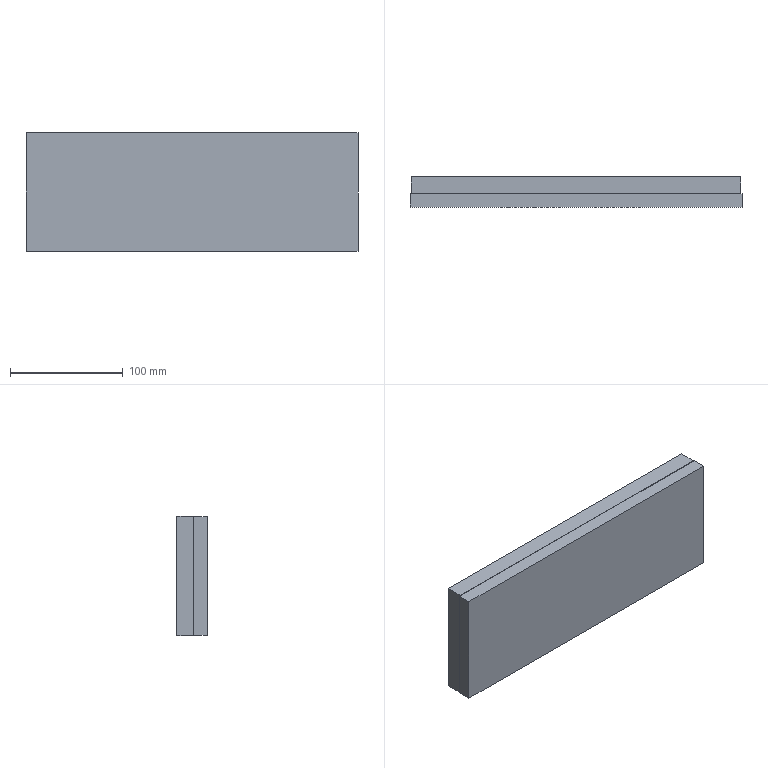NC program | NX | posted with a generic post | part box 295 x 27 x 106 mm
Lines 1 to 1810 of 7486, first 1519 of 1788 lines:
N10 G17 G21 G94 G90
(DRILLING , TOOL : DK-D8点孔)
N12 T04 M6
N14 G53
N16 G17 G0 G90 X102. Y-38.5 S2000 M3
N18 G43 Z20. H4
N20 G94 G81 G99 Z-3. F200. R3.
N22 Y0.
N24 Y38.5
N26 X-117. Y38.616
N28 Y0.
N30 G80
N32 G0 X-117. Y0. Z20.
N34 M5
(DRILLING_COPY , TOOL : D05钻头)
N36 T05 M6
N38 G53
N40 G17 G0 G90 X102. Y-38.5 S2000 M3
N42 G43 Z20. H5
N44 G94 G81 G99 Z-14. F200. R3.
N46 Y38.5
N48 X-117. Y0.
N50 G80
N52 G0 X-117. Y0. Z20.
(DRILLING_COPY_1 , TOOL : D05钻头)
N54 Y38.616
N56 G81 Z-7. F200. R3.
N58 X102. Y0.
N60 G80
N62 G0 X102. Y0. Z20.
N64 M5
(FLOOR_WALL_1 , TOOL : D63光面)
N66 T01 M6
N68 G54
N70 G17 G0 G90 X222.5 Y-30.25 S4000 M3
N72 G43 Z4.525 H1
N74 G94 G1 Z1.525 F1000.
N76 X212.5
N78 X-135.5
N80 Y-1.725
N82 X212.5
N84 Y26.8
N86 X-135.5
N88 X-145.5
N90 Z4.525
N92 G0 Z5.
N94 X222.5 Y-30.25
N96 Z4.05
N98 G1 Z1.05
N100 X212.5
N102 X-135.5
N104 Y-1.725
N106 X212.5
N108 Y26.8
N110 X-135.5
N112 X-145.5
N114 Z4.05
N116 G0 Z5.
N118 X222.5 Y-30.25
N120 Z3.575
N122 G1 Z0.575
N124 X212.5
N126 X-135.5
N128 Y-1.725
N130 X212.5
N132 Y26.8
N134 X-135.5
N136 X-145.5
N138 Z3.575
N140 G0 Z5.
N142 X222.5 Y-30.25
N144 Z3.1
N146 G1 Z0.1
N148 X212.5
N150 X-135.5
N152 Y-1.725
N154 X212.5
N156 Y26.8
N158 X-135.5
N160 X-145.5
N162 Z3.1
N164 G0 Z5.
(FLOOR_WALL_1_COPY , TOOL : D63光面)
N166 X222.5 Y-30.25
N168 Z3.
N170 G1 Z0. F800.
N172 X212.5
N174 X-135.5
N176 X-145.5
N178 Z3.
N180 G0 Z5.
N182 X222.5 Y-1.725
N184 Z3.
N186 G1 Z0.
N188 X212.5
N190 X-135.5
N192 X-145.5
N194 Z3.
N196 G0 Z5.
N198 X222.5 Y26.8
N200 Z3.
N202 G1 Z0.
N204 X212.5
N206 X-135.5
N208 X-145.5
N210 Z3.
N212 G0 Z5.
N214 M5
(ADAPTIVE_MILLING_2 , TOOL : D8R0波刀)
N216 T02 M6
N218 G54
N220 G17 G0 G90 X-0.64 Y-31.763 S6500 M3
N222 G43 Z3. H2
N224 Z-1.
N226 G94 G1 X-0.636 Y-31.913 Z-1.937 F3000.
N228 X-0.632 Y-32.063 Z-2.308
N230 X-0.629 Y-32.213 Z-2.58
N232 X-0.625 Y-32.363 Z-2.8
N234 X-0.622 Y-32.513 Z-2.984
N236 X-0.618 Y-32.663 Z-3.142
N238 X-0.614 Y-32.813 Z-3.28
N240 X-0.611 Y-32.963 Z-3.4
N242 X-0.607 Y-33.113 Z-3.505
N244 X-0.604 Y-33.263 Z-3.598
N246 X-0.6 Y-33.413 Z-3.679
N248 X-0.597 Y-33.563 Z-3.75
N250 X-0.593 Y-33.713 Z-3.81
N252 X-0.589 Y-33.863 Z-3.862
N254 X-0.586 Y-34.013 Z-3.905
N256 X-0.582 Y-34.163 Z-3.939
N258 X-0.579 Y-34.313 Z-3.966
N260 X-0.575 Y-34.463 Z-3.985
N262 X-0.572 Y-34.612 Z-3.996
N264 X-0.568 Y-34.762 Z-4.
N266 X-0.537 Y-36.079
N268 G3 X-0.018 Y-36.814 R0.809
N270 X2.31 Y-37.159 R6.531
N272 X9.781 Y-36.066 R28.433
N274 X-24.985 Y27.795 R-37.373
N276 X-2.157 Y-37.311 R37.372
N278 X2.194 Y-37.672 R43.722
N280 X11.765 Y-36.041 R30.956
N282 X-4.119 Y-37.689 R-37.917
N284 X1.568 Y-38.195 R64.185
N286 X12.804 Y-36.26 R32.077
N288 X-27.631 Y-26.756 R-38.462
N290 X-4.06 Y-38.264 R38.776
N292 X3.503 Y-38.698 R40.785
N294 X17.75 Y-34.728 R35.763
N296 X-6.551 Y-38.451 R-39.006
N298 X2.274 Y-39.275 R48.648
N300 X16.915 Y-35.745 R35.636
N302 X-8.562 Y-38.612 R-39.552
N304 X2.471 Y-39.813 R47.92
N306 X18.487 Y-35.574 R36.733
N308 X-9.82 Y-38.875 R-40.098
N310 X2.534 Y-40.354 R47.189
N312 X19.934 Y-35.412 R37.65
N314 X-12.93 Y-38.532 R-40.645
N316 X3.011 Y-40.882 R46.391
N318 X21.575 Y-35.08 R38.598
N320 X-14.242 Y-38.65 R-41.192
N322 X3.269 Y-41.415 R46.135
N324 X22.879 Y-34.9 R39.38
N326 X-16.168 Y-38.48 R-41.74
N328 X3.45 Y-41.951 R46.073
N330 X24.323 Y-34.582 R40.151
N332 X-22.838 Y-35.59 R-42.288
N334 X-5.541 Y-42.007 R44.372
N336 X12.726 Y-40.859 R40.542
N338 X30.019 Y30.546 R42.768
N340 X-10.726 Y-41.487 R-42.838
N342 X4.932 Y-42.938 R45.348
N344 X27.736 Y-33.351 R41.762
N346 X-25.127 Y-35.369 R-43.386
N348 X-6.183 Y-43.03 R45.145
N350 X13.838 Y-41.657 R41.94
N352 X28.359 Y33.547 R43.874
N354 X-12.172 Y-42.23 R-43.938
N356 X5.279 Y-44.005 R46.213
N358 X29.603 Y-33.196 R43.016
N360 X-25.798 Y-36.241 R-44.487
N362 X-5.777 Y-44.22 R46.403
N364 X27.412 Y-35.722 R43.096
N366 X-44.99 Y2.184 R-45.037
N368 X-11.568 Y-43.555 R45.156
N370 X7.194 Y-44.88 R46.327
N372 X33.283 Y-31.143 R44.508
N374 X-25.316 Y-37.913 R-45.59
N376 X5.449 Y-45.645 R47.884
N378 X31.755 Y-33.465 R44.799
N380 X-27.179 Y-37.286 R-46.142
N382 X-5.09 Y-46. R48.096
N384 G1 X6.219 Y-45.986
N386 G3 X14.527 Y-44.318 R34.532
N388 X46.383 Y-5.465 R46.527
N390 X-15.069 Y-44.212 R-46.699
N392 X-8.455 Y-46. R49.755
N394 G1 X-5.08
N396 G3 X-4.388 Y-45.602 R0.801
N398 G1 X-4.255 Y-45.373
N400 X-3.543 Y-44.154 Z-3.911
N402 X-3.437 Y-44.025 Z-3.9
N404 G2 X-2.882 Y-43.802 R0.805 F15000.
N406 G1 X3.663
N408 G2 X4.205 Y-44.014 R0.805
N410 G1 X4.354 Y-44.199 Z-3.915 F3000.
N412 X4.473 Y-44.405 Z-3.93
N414 X5.027 Y-45.358 Z-4.
N416 X5.236 Y-45.7
N418 G3 X5.86 Y-46. R0.802
N420 X9.542 Y-45.959 R53.454
N422 X16.091 Y-44.366 R28.941
N424 X46.805 Y-6.514 R47.069
N426 X-15.705 Y-44.577 R-47.252
N428 X-10.965 Y-46. R48.51
N430 G1 X-8.415
N432 G3 X-7.724 Y-45.602 R0.801
N434 G1 X-7.59 Y-45.373
N436 X-6.878 Y-44.154 Z-3.911
N438 X-6.772 Y-44.025 Z-3.9
N440 G2 X-6.217 Y-43.802 R0.805 F15000.
N442 G1 X6.663
N444 G2 X7.205 Y-44.014 R0.805
N446 G1 X7.354 Y-44.199 Z-3.915 F3000.
N448 X7.473 Y-44.405 Z-3.93
N450 X8.027 Y-45.358 Z-4.
N452 X8.236 Y-45.7
N454 G3 X8.86 Y-46. R0.802
N456 X11.773 Y-45.955 R34.063
N458 X17.472 Y-44.43 R24.517
N460 X44.102 Y-18.439 R47.422
N462 X-16.965 Y-44.702 R-47.803
N464 X-13.07 Y-46. R37.021
N466 G1 X-10.895
N468 G3 X-10.203 Y-45.602 R0.801
N470 G1 X-10.07 Y-45.373
N472 X-9.357 Y-44.154 Z-3.911
N474 X-9.251 Y-44.025 Z-3.9
N476 G2 X-8.697 Y-43.802 R0.805 F15000.
N478 G1 X8.913
N480 G2 X9.455 Y-44.014 R0.805
N482 G1 X9.604 Y-44.199 Z-3.915 F3000.
N484 X9.723 Y-44.405 Z-3.93
N486 X10.277 Y-45.358 Z-4.
N488 X10.486 Y-45.7
N490 G3 X11.11 Y-46. R0.802
N492 X13.779 Y-45.937 R22.187
N494 X19.058 Y-44.372 R22.68
N496 X41.485 Y-24.837 R47.674
N498 X-19.274 Y-44.355 R-48.359
N500 X-14.965 Y-45.993 R45.527
N502 G1 X-13.028 Y-46.
N504 G3 X-12.336 Y-45.602 R0.801
N506 G1 X-12.203 Y-45.373
N508 X-11.49 Y-44.154 Z-3.911
N510 X-11.384 Y-44.025 Z-3.9
N512 G2 X-10.83 Y-43.802 R0.805 F15000.
N514 G1 X10.863
N516 G2 X11.405 Y-44.014 R0.805
N518 G1 X11.554 Y-44.199 Z-3.915 F3000.
N520 X11.673 Y-44.405 Z-3.93
N522 X12.227 Y-45.358 Z-4.
N524 X12.436 Y-45.7
N526 G3 X13.06 Y-46. R0.802
N528 X15.541 Y-45.918 R16.436
N530 X20.714 Y-44.233 R21.576
N532 X41.135 Y-26.451 R48.024
N534 X-22.042 Y-43.665 R-48.913
N536 X-16.667 Y-45.987 R47.044
N538 G1 X-14.853 Y-46.
N540 G3 X-14.162 Y-45.602 R0.801
N542 G1 X-14.028 Y-45.373
N544 X-13.316 Y-44.154 Z-3.911
N546 X-13.21 Y-44.025 Z-3.9
N548 G2 X-12.655 Y-43.802 R0.805 F15000.
N550 G1 X12.513
N552 G2 X13.055 Y-44.014 R0.805
N554 G1 X13.204 Y-44.199 Z-3.915 F3000.
N556 X13.323 Y-44.405 Z-3.93
N558 X13.877 Y-45.358 Z-4.
N560 X14.086 Y-45.7
N562 G3 X14.71 Y-46. R0.802
N564 X17.063 Y-45.913 R14.512
N566 X21.88 Y-44.273 R19.665
N568 X38.981 Y-30.441 R47.796
N570 X-36.979 Y-32.851 R-49.466
N572 X-18.283 Y-45.968 R49.568
N574 G1 X-18.111 Y-46.
N576 X-16.536
N578 G3 X-15.844 Y-45.602 R0.801
N580 G1 X-15.711 Y-45.373
N582 X-14.998 Y-44.154 Z-3.911
N584 X-14.892 Y-44.025 Z-3.9
N586 G2 X-14.338 Y-43.802 R0.805 F15000.
N588 G1 X14.013
N590 G2 X14.555 Y-44.014 R0.805
N592 G1 X14.704 Y-44.199 Z-3.915 F3000.
N594 X14.823 Y-44.405 Z-3.93
N596 X15.377 Y-45.358 Z-4.
N598 X15.586 Y-45.7
N600 G3 X16.21 Y-46. R0.802
N602 X18.466 Y-45.911 R13.161
N604 X23.197 Y-44.215 R18.555
N606 X38.232 Y-32.244 R47.648
N608 X-48.568 Y11.987 R-50.021
N610 X-19.728 Y-45.963 R50.016
N612 G1 X-19.532 Y-46.
N614 X-18.107
N616 G3 X-17.416 Y-45.602 R0.801
N618 G1 X-17.282 Y-45.373
N620 X-16.57 Y-44.154 Z-3.911
N622 X-16.464 Y-44.025 Z-3.9
N624 G2 X-15.91 Y-43.802 R0.805 F15000.
N626 G1 X15.438
N628 G2 X15.98 Y-44.014 R0.805
N630 G1 X16.129 Y-44.199 Z-3.915 F3000.
N632 X16.248 Y-44.405 Z-3.93
N634 X16.802 Y-45.358 Z-4.
N636 X17.011 Y-45.7
N638 G3 X17.635 Y-46. R0.802
N640 X19.847 Y-45.897 R11.416
N642 X24.425 Y-44.17 R17.851
N644 X37.819 Y-33.571 R47.316
N646 X-47.783 Y16.586 R-50.576
N648 X-21.112 Y-45.95 R50.554
N650 G1 X-20.886 Y-46.
N652 X-19.461
N654 G3 X-18.769 Y-45.602 R0.801
N656 G1 X-18.636 Y-45.373
N658 X-17.923 Y-44.154 Z-3.911
N660 X-17.817 Y-44.025 Z-3.9
N662 G2 X-17.263 Y-43.802 R0.805 F15000.
N664 G1 X16.788
N666 G2 X17.33 Y-44.014 R0.805
N668 G1 X17.479 Y-44.199 Z-3.915 F3000.
N670 X17.598 Y-44.405 Z-3.93
N672 X18.152 Y-45.358 Z-4.
N674 X18.361 Y-45.7
N676 G3 X18.985 Y-46. R0.802
N678 X21.101 Y-45.894 R10.329
N680 X25.593 Y-44.133 R17.112
N682 X37.74 Y-34.49 R46.878
N684 X-47.208 Y19.651 R-51.132
N686 X-22.637 Y-45.843 R51.112
N688 X-22.161 Y-46. R2.079
N690 G1 X-20.886
N692 G3 X-20.194 Y-45.602 R0.801
N694 G1 X-20.061 Y-45.373
N696 X-19.348 Y-44.154 Z-3.911
N698 X-19.242 Y-44.025 Z-3.9
N700 G2 X-18.688 Y-43.802 R0.805 F15000.
N702 G1 X18.063
N704 G2 X18.605 Y-44.014 R0.805
N706 G1 X18.754 Y-44.199 Z-3.915 F3000.
N708 X18.873 Y-44.405 Z-3.93
N710 X19.427 Y-45.358 Z-4.
N712 X19.636 Y-45.7
N714 G3 X20.26 Y-46. R0.802
N716 X22.448 Y-45.859 R9.051
N718 X26.971 Y-43.956 R17.491
N720 X39.062 Y-33.842 R47.291
N722 X-44.619 Y26.098 R-51.688
N724 X-23.859 Y-45.841 R51.648
N726 X-23.378 Y-46. R1.84
N728 G1 X-22.103
N730 G3 X-21.411 Y-45.602 R0.801
N732 G1 X-21.278 Y-45.373
N734 X-20.566 Y-44.154 Z-3.911
N736 X-20.46 Y-44.025 Z-3.9
N738 G2 X-19.905 Y-43.802 R0.805 F15000.
N740 G1 X19.263
N742 G2 X19.805 Y-44.014 R0.805
N744 G1 X19.954 Y-44.199 Z-3.915 F3000.
N746 X20.073 Y-44.405 Z-3.93
N748 X20.627 Y-45.358 Z-4.
N750 X20.836 Y-45.7
N752 G3 X21.46 Y-46. R0.802
N754 X23.729 Y-45.823 R8.292
N756 X28.209 Y-43.828 R17.724
N758 X39.71 Y-33.943 R47.328
N760 X5.807 Y51.931 R52.243
N762 G1 X5.155 Y52.
N764 G3 X-4.598 Y51.98 R546.7
N766 X-17.616 Y49.192 R47.297
N768 X-25.178 Y-45.767 R52.235
N770 X-24.553 Y-46. R2.101
N772 G1 X-23.353
N774 G3 X-22.661 Y-45.602 R0.801
N776 G1 X-22.528 Y-45.373
N778 X-21.816 Y-44.154 Z-3.911
N780 X-21.71 Y-44.025 Z-3.9
N782 G2 X-21.155 Y-43.802 R0.805 F15000.
N784 G1 X20.388
N786 G2 X20.93 Y-44.014 R0.805
N788 G1 X21.079 Y-44.199 Z-3.915 F3000.
N790 X21.198 Y-44.405 Z-3.93
N792 X21.752 Y-45.358 Z-4.
N794 X21.961 Y-45.7
N796 G3 X22.585 Y-46. R0.802
N798 X24.742 Y-45.84 R8.09
N800 X29.096 Y-43.888 R16.528
N802 X39.65 Y-34.863 R46.348
N804 X9.202 Y52. R52.793
N806 G1 X5.152
N808 G3 X4.398 Y51.572 R0.881
N810 X4.303 Y50.877 Z-3.954 R0.925
N812 G1 X4.465 Y50.034 Z-3.9
N814 X22.602 Y-44.019 F15000.
N816 X22.728 Y-44.688 Z-3.943 F3000.
N818 X22.866 Y-45.356 Z-3.986
N820 X22.901 Y-45.457 Z-3.993
N822 X22.945 Y-45.555 Z-4.
N824 G3 X23.71 Y-46. R0.881
N826 X27.428 Y-45.279 R7.573
N828 X33.328 Y-41.608 R28.376
N830 X50.051 Y-18.525 R52.578
N832 X11.974 Y52. R53.356
N834 G1 X9.199
N836 G3 X8.447 Y51.576 R0.881
N838 X8.342 Y50.907 Z-3.956 R0.924
N840 G1 X8.483 Y50.034 Z-3.9
N842 X23.691 Y-44.019 F15000.
N844 X23.797 Y-44.693 Z-3.943 F3000.
N846 X23.915 Y-45.365 Z-3.986
N848 X23.999 Y-45.561 Z-4.
N850 G3 X24.76 Y-46. R0.881
N852 X28.395 Y-45.291 R7.314
N854 X33.998 Y-41.771 R26.927
N856 X35.895 Y-40.179 R46.544
N858 G1 X36.487 Y-39.156
N860 X37.1 Y-38.479
N862 X39.723 Y-35.973
N864 X42.159 Y-33.324
N866 G3 X45.359 Y-29.111 R48.612
N868 X35.635 Y40.461 R53.807
N870 X14.298 Y51.992 R53.978
N872 G1 X11.974 Y52.
N874 G3 X11.222 Y51.579 R0.881
N876 X11.113 Y50.921 Z-3.957 R0.925
N878 G1 X11.241 Y50.034 Z-3.9
N880 X24.763 Y-44.019 F15000.
N882 X24.856 Y-44.689 Z-3.943 F3000.
N884 X24.963 Y-45.356 Z-3.986
N886 X25.051 Y-45.564 Z-4.
N888 G3 X25.81 Y-46. R0.881
N890 X29.233 Y-45.349 R6.954
N892 X35.515 Y-41.193 R25.236
N894 X35.746 Y-40.813 R1.186
N896 G1 X36.025 Y-39.957
N898 G3 X35.608 Y-38.911 R0.88
N900 X34.651 Y-38.984 Z-3.936 R0.9
N902 G1 X34.176 Y-39.291 Z-3.9
N904 X26.865 Y-44.02 F15000.
N906 X26.53 Y-44.234 Z-3.925 F3000.
N908 X26.203 Y-44.46 Z-3.95
N910 G3 X25.906 Y-45.158 Z-4. R0.892
N912 X26.785 Y-46. R0.88
N914 X30.258 Y-45.316 R6.88
N916 X35.189 Y-42.122 R19.897
N918 X35.686 Y-41.379 R1.534
N920 G1 X35.769 Y-40.742
N922 G3 X35.348 Y-39.693 R0.88
N924 X34.394 Y-39.769 Z-3.936 R0.901
N926 G1 X33.917 Y-40.079 Z-3.9
N928 X27.839 Y-44.02 F15000.
N930 X27.504 Y-44.234 Z-3.925 F3000.
N932 X27.178 Y-44.461 Z-3.95
N934 G3 X26.881 Y-45.159 Z-4. R0.892
N936 X27.76 Y-46. R0.88
N938 X31.278 Y-45.277 R6.809
N940 X35.14 Y-42.756 R14.37
N942 X35.65 Y-41.892 R1.486
N944 G1 X35.689 Y-41.348
N946 G3 X35.193 Y-40.461 R0.881
N948 X34.278 Y-40.554 Z-3.939 R0.904
N950 G1 X33.761 Y-40.882 Z-3.9
N952 X28.822 Y-44.022 F15000.
N954 X28.486 Y-44.233 Z-3.925 F3000.
N956 X28.158 Y-44.456 Z-3.95
N958 G3 X27.856 Y-45.152 Z-4. R0.892
N960 X28.735 Y-46. R0.88
N962 X32.024 Y-45.353 R6.521
N964 X35.191 Y-43.257 R10.182
N966 X35.65 Y-42.426 R1.468
N968 G1 Y-41.826
N970 G3 X35.126 Y-41.022 R0.881
N972 X34.224 Y-41.132 Z-3.94 R0.905
N974 G1 X33.7 Y-41.473 Z-3.9
N976 X29.786 Y-44.021 F15000.
N978 X29.452 Y-44.235 Z-3.925 F3000.
N980 X29.126 Y-44.462 Z-3.95
N982 G3 X28.831 Y-45.162 Z-4. R0.892
N984 X29.71 Y-46. R0.88
N986 X33.188 Y-45.213 R6.365
N988 X35.438 Y-43.478 R6.365
N990 X35.65 Y-42.96 R1.059
N992 G1 Y-42.36
N994 G3 X35.106 Y-41.546 R0.881
N996 X34.224 Y-41.666 Z-3.941 R0.907
N998 G1 X33.685 Y-42.023 Z-3.9
N1000 X30.675 Y-44.021 F15000.
N1002 X30.344 Y-44.238 Z-3.925 F3000.
N1004 X30.02 Y-44.467 Z-3.95
N1006 G3 X29.732 Y-45.17 Z-4. R0.892
N1008 X30.61 Y-46. R0.88
N1010 X35.382 Y-44.05 R5.855
N1012 X35.65 Y-43.459 R1.148
N1014 G1 Y-42.934
N1016 G3 X35.104 Y-42.12 R0.881
N1018 X34.22 Y-42.243 Z-3.941 R0.907
N1020 G1 X33.685 Y-42.602 Z-3.9
N1022 X31.57 Y-44.021 F15000.
N1024 X31.239 Y-44.239 Z-3.925 F3000.
N1026 X30.917 Y-44.47 Z-3.95
N1028 G3 X30.632 Y-45.175 Z-4. R0.892
N1030 X31.51 Y-46. R0.88
N1032 X35.276 Y-44.618 R4.805
N1034 X35.65 Y-43.91 R1.213
N1036 G1 Y-43.385
N1038 G3 X35.091 Y-42.566 R0.881
N1040 X34.196 Y-42.714 Z-3.94 R0.905
N1042 G1 X33.685 Y-43.078 Z-3.9
N1044 X32.362 Y-44.02 F15000.
N1046 X32.039 Y-44.248 Z-3.925 F3000.
N1048 X31.724 Y-44.487 Z-3.95
N1050 G3 X31.459 Y-45.201 Z-4. R0.892
N1052 X32.335 Y-46. R0.88
N1054 X35.152 Y-45.116 R3.861
N1056 X35.65 Y-44.299 R1.26
N1058 G1 Y-43.849
N1060 G3 X35.079 Y-43.025 R0.881
N1062 X34.178 Y-43.193 Z-3.939 R0.905
N1064 G1 X33.685 Y-43.565 Z-3.9
N1066 X33.083 Y-44.02 F15000.
N1068 X32.765 Y-44.256 Z-3.925 F3000.
N1070 X32.457 Y-44.504 Z-3.95
N1072 G3 X32.212 Y-45.225 Z-4. R0.892
N1074 X33.085 Y-46. R0.88
N1076 X35.471 Y-45.1 R2.855
N1078 X35.65 Y-44.246 R1.279
N1080 X35.06 Y-43.415 R0.88
N1082 X34.158 Y-43.608 Z-3.939 R0.904
N1084 G1 X33.683 Y-43.991 Z-3.9
N1086 X33.646 Y-44.021 F15000.
N1088 X33.337 Y-44.267 Z-3.925 F3000.
N1090 X33.037 Y-44.525 Z-3.95
N1092 G3 X32.816 Y-45.254 Z-4. R0.892
N1094 X33.685 Y-46. R0.88
N1096 X35.499 Y-45.316 R2.119
N1098 X35.65 Y-44.588 R1.121
N1100 X34.205 Y-43.914 R0.88
N1102 G1 X33.57 Y-44.446
N1104 G3 X34.135 Y-46. R0.88
N1106 X35.49 Y-45.512 R1.548
N1108 X35.65 Y-44.844 R1.031
N1110 X34.13 Y-44.241 R0.88
N1112 G1 X33.952 Y-44.427
N1114 X33.784 Y-44.623
N1116 G3 X34.51 Y-46. R0.88
N1118 X35.505 Y-45.611 R1.036
N1120 X35.65 Y-45.013 R1.023
N1122 X33.882 Y-44.715 R0.91
N1124 X34.887 Y-45.992 R0.956
N1126 X35.637 Y-45.274 R0.818
N1128 X35.256 Y-44.5 R0.801
N1130 G1 X35.033 Y-44.365
N1132 X33.681 Y-43.549 Z-3.9
N1134 G2 X33.306 Y-43.269 R1.313 F15000.
N1136 X33.126 Y-42.763 R0.807
N1138 G1 X33.124 Y-42.107
N1140 X33.136 Y-41.451
N1142 G2 X33.49 Y-39.872 R5.184
N1144 G1 X33.98 Y-38.668
N1146 G2 X35.738 Y-36.046 R9.597
N1148 G1 X40.398 Y-31.106
N1150 G2 X41.178 Y-30.88 R0.801
N1152 G1 X41.507 Y-30.964
N1154 X43.037 Y-31.355 Z-4. F3000.
N1156 G3 X43.95 Y-31.106 R0.832
N1158 G1 X44.42 Y-30.522
N1160 X46.494 Y-27.58
N1162 X48.374 Y-24.51
N1164 G3 X50.204 Y-20.982 R99.505
N1166 X53.558 Y-10.091 R48.023
N1168 X16.265 Y51.991 R54.496
N1170 G1 X14.165 Y52.
N1172 G3 X13.375 Y51.508 R0.881
N1174 X13.407 Y50.667 Z-3.945 R0.912
N1176 G1 X13.713 Y50.034 Z-3.9
N1178 X48.029 Y-20.917 F15000.
N1180 X48.379 Y-21.625 Z-3.95 F3000.
N1182 G3 X49.009 Y-22.052 Z-4. R0.879
N1184 X49.913 Y-21.591 R0.881
N1186 X51.519 Y-18.038 R227.445
N1188 G1 X52.771 Y-14.663
N1190 X53.833 Y-11.084
N1192 G3 X55.069 Y0.116 R46.882
N1194 X18.037 Y51.99 R55.093
N1196 G1 X16.162 Y52.
N1198 G3 X15.358 Y51.478 R0.881
N1200 X15.442 Y50.609 Z-3.942 R0.908
N1202 G1 X15.781 Y50.035 Z-3.9
N1204 X51.791 Y-11.035 F15000.
N1206 X51.995 Y-11.386 Z-3.926 F3000.
N1208 X52.212 Y-11.73 Z-3.952
N1210 G3 X52.877 Y-12.058 Z-4. R0.892
N1212 X53.74 Y-11.43 R0.88
N1214 G1 X54.61 Y-7.706
N1216 X55.187 Y-4.153
N1218 G3 X55.545 Y-0.233 R125.615
N1220 X54.721 Y9.98 R46.585
N1222 X19.729 Y51.975 R55.681
N1224 G1 X19.581 Y52.
N1226 X17.931
N1228 G3 X17.112 Y51.443 R0.881
N1230 X17.258 Y50.548 Z-3.94 R0.906
N1232 G1 X17.62 Y50.035 Z-3.9
N1234 X53.529 Y-0.749 F15000.
N1236 X53.756 Y-1.075 Z-3.925 F3000.
N1238 X53.996 Y-1.392 Z-3.95
N1240 G3 X54.704 Y-1.661 Z-4. R0.892
N1242 X55.507 Y-0.869 R0.88
N1244 X55.649 Y3.028 R227.044
N1246 G1 X55.531 Y6.625
N1248 G3 X55.042 Y10.993 R61.389
N1250 X49.573 Y26.395 R53.186
N1252 X21.264 Y51.967 R56.125
N1254 G1 X21.088 Y52.
N1256 X19.513
N1258 G3 X18.678 Y51.399 R0.88
N1260 X18.888 Y50.496 Z-3.938 R0.903
N1262 G1 X19.277 Y50.033 Z-3.9
N1264 X53.252 Y9.614 F15000.
N1266 X53.504 Y9.309 Z-3.925 F3000.
N1268 X53.768 Y9.015 Z-3.95
N1270 G3 X54.501 Y8.808 Z-4. R0.892
N1272 X55.226 Y9.761 R0.88
N1274 X54.599 Y13.76 R78.936
N1276 G1 X53.789 Y17.268
N1278 G3 X52.419 Y21.563 R56.849
N1280 X41.278 Y38.903 R55.168
N1282 X22.691 Y51.965 R56.283
N1284 G1 X22.506 Y52.
N1286 X21.081
N1288 G3 X20.232 Y51.351 R0.88
N1290 X20.508 Y50.448 Z-3.937 R0.902
N1292 G1 X20.92 Y50.033 Z-3.9
N1294 X50.979 Y19.754 F15000.
N1296 X51.263 Y19.465 Z-3.926 F3000.
N1298 X51.557 Y19.185 Z-3.951
N1300 G3 X52.284 Y19.032 Z-4. R0.892
N1302 X52.928 Y20.142 R0.88
N1304 G1 X52.754 Y20.716
N1306 X51.498 Y24.089
N1308 X50.027 Y27.375
N1310 X48.268 Y30.685
N1312 G3 X40.564 Y40.446 R50.585
N1314 X24.08 Y51.952 R56.36
N1316 G1 X23.86 Y52.
N1318 X22.435
N1320 G3 X21.571 Y51.288 R0.88
N1322 X21.924 Y50.4 Z-3.936 R0.901
N1324 G1 X22.361 Y50.034 Z-3.9
N1326 X46.498 Y29.788 F15000.
N1328 X46.851 Y29.487 Z-3.929 F3000.
N1330 X47.214 Y29.199 Z-3.959
N1332 G3 X47.841 Y29.085 Z-4. R0.901
N1334 X48.453 Y30.36 R0.88
N1336 G1 X46.464 Y33.626
N1338 X44.386 Y36.566
N1340 X42.123 Y39.365
N1342 G3 X38.615 Y43.022 R58.468
N1344 X25.384 Y51.946 R53.953
N1346 G1 X25.146 Y52.
N1348 X23.796
N1350 G3 X22.918 Y51.18 R0.88
N1352 X23.379 Y50.342 Z-3.936 R0.901
N1354 G1 X23.857 Y50.033 Z-3.9
N1356 X37.937 Y40.947 F15000.
N1358 X38.449 Y40.612 Z-3.939 F3000.
N1360 X38.969 Y40.29 Z-3.978
N1362 X39.137 Y40.234 Z-3.989
N1364 X39.312 Y40.208 Z-4.
N1366 G3 X39.99 Y41.683 R0.88
N1368 X37.1 Y44.479 R80.633
N1370 X33.037 Y48.118 R20.123
N1372 X26.623 Y51.944 R44.006
N1374 G1 X26.378 Y52.
N1376 X25.103
N1378 G3 X24.223 Y51.146 R0.88
N1380 X24.71 Y50.329 Z-3.937 R0.901
N1382 G1 X25.203 Y50.032 Z-3.9
N1384 X34.69 Y44.311 F15000.
N1386 X35.034 Y44.101 Z-3.926 F3000.
N1388 X35.386 Y43.902 Z-3.951
N1390 G3 X36.132 Y43.933 Z-4. R0.892
N1392 X36.487 Y45.156 R0.88
N1394 X34.328 Y47.71 R8.269
N1396 X27.791 Y51.947 R33.543
N1398 G1 X27.556 Y52.
N1400 X26.356
N1402 G3 X25.478 Y51.177 R0.88
N1404 X25.941 Y50.34 Z-3.936 R0.901
N1406 G1 X26.421 Y50.033 Z-3.9
N1408 X34.296 Y44.993 F15000.
N1410 X34.637 Y44.771 Z-3.926 F3000.
N1412 X34.987 Y44.561 Z-3.952
N1414 G3 X35.726 Y44.568 Z-4. R0.892
N1416 X36.111 Y45.805 R0.88
N1418 G1 X35.742 Y46.581
N1420 G3 X33.4 Y49.038 R10.182
N1422 X28.959 Y51.926 R26.492
N1424 G1 X28.669 Y52.
N1426 X27.544
N1428 G3 X26.669 Y51.215 R0.88
N1430 X27.098 Y50.358 Z-3.936 R0.901
N1432 G1 X27.563 Y50.033 Z-3.9
N1434 X34.1 Y45.472 F15000.
N1436 X34.423 Y45.243 Z-3.925 F3000.
N1438 X34.755 Y45.027 Z-3.95
N1440 G3 X35.515 Y45.016 Z-4. R0.892
N1442 X35.982 Y46.088 R0.88
N1444 X34.509 Y48.575 R5.336
N1446 X29.94 Y51.949 R18.182
N1448 G1 X29.711 Y52.
N1450 X28.661
N1452 G3 X27.789 Y51.236 R0.88
N1454 X28.197 Y50.369 Z-3.936 R0.901
N1456 G1 X28.654 Y50.033 Z-3.9
N1458 X33.86 Y46.21 F15000.
N1460 X34.177 Y45.974 Z-3.925 F3000.
N1462 X34.503 Y45.749 Z-3.95
N1464 G3 X35.264 Y45.721 Z-4. R0.892
N1466 X35.75 Y46.801 R0.88
N1468 X34.975 Y48.513 R3.557
N1470 X30.879 Y51.949 R12.983
N1472 G1 X30.648 Y52.
N1474 X29.673
N1476 G3 X28.808 Y51.28 R0.88
N1478 X29.17 Y50.394 Z-3.936 R0.901
N1480 G1 X29.61 Y50.034 Z-3.9
N1482 X33.774 Y46.619 F15000.
N1484 X34.084 Y46.361 Z-3.926 F3000.
N1486 X34.402 Y46.116 Z-3.951
N1488 G3 X35.147 Y46.04 Z-4. R0.892
N1490 X35.73 Y46.963 R0.88
N1492 X34.887 Y49.128 R3.846
N1494 X31.778 Y51.922 R10.327
N1496 G1 X31.48 Y52.
N1498 X30.58
N1500 G3 X29.722 Y51.313 R0.88
N1502 X30.045 Y50.418 Z-3.936 R0.901
N1504 G1 X30.472 Y50.034 Z-3.9
N1506 X33.723 Y47.11 F15000.
N1508 X34.018 Y46.841 Z-3.925 F3000.
N1510 X34.322 Y46.584 Z-3.951
N1512 G3 X35.071 Y46.478 Z-4. R0.892
N1514 X35.683 Y47.41 R0.88
N1516 X34.849 Y49.698 R3.946
N1518 X32.489 Y51.927 R7.588
N1520 G1 X32.199 Y52.
N1522 X31.449
N1524 G3 X30.6 Y51.349 R0.88
N1526 X30.879 Y50.446 Z-3.937 R0.902
N1528 G1 X31.291 Y50.033 Z-3.9
N1530 X33.674 Y47.649 F15000.
N1532 X33.955 Y47.365 Z-3.925 F3000.
N1534 X34.246 Y47.09 Z-3.951
N1536 G3 X34.985 Y46.944 Z-4. R0.892
N1538 X35.65 Y47.797 R0.88
N1540 X34.945 Y50.089 R3.639
N1542 X33.095 Y51.933 R5.492
N1544 G1 X32.809 Y52.
N1546 X32.134
N1548 G3 X31.292 Y51.374 R0.88
N1550 X31.536 Y50.47 Z-3.938 R0.903
N1552 G1 X31.937 Y50.033 Z-3.9
N1554 X33.67 Y48.144 F15000.
N1556 X33.938 Y47.849 Z-3.925 F3000.
N1558 X34.216 Y47.563 Z-3.951
N1560 G3 X34.951 Y47.386 Z-4. R0.892
N1562 X35.65 Y48.247 R0.88
N1564 X34.887 Y50.704 R3.718
N1566 X33.631 Y51.93 R3.874
N1568 X32.741 Y52. R2.429
N1570 X31.904 Y51.391 R0.88
N1572 X32.124 Y50.488 Z-3.938 R0.903
N1574 G1 X32.517 Y50.033 Z-3.9
N1576 X33.671 Y48.698 F15000.
N1578 X33.928 Y48.396 Z-3.925 F3000.
N1580 X34.197 Y48.104 Z-3.95
N1582 G3 X34.93 Y47.907 Z-4. R0.892
N1584 X35.65 Y48.772 R0.88
N1586 X34.097 Y51.92 R3.515
N1588 X33.271 Y52. R2.019
N1590 X32.438 Y51.405 R0.88
N1592 X32.64 Y50.502 Z-3.939 R0.904
N1594 G1 X33.025 Y50.033 Z-3.9
N1596 X33.671 Y49.248 F15000.
N1598 X33.92 Y48.941 Z-3.925 F3000.
N1600 X34.181 Y48.643 Z-3.95
N1602 G3 X34.911 Y48.429 Z-4. R0.892
N1604 X35.65 Y49.297 R0.88
N1606 X34.506 Y51.897 R2.894
N1608 X33.773 Y52. R1.364
N1610 X32.947 Y51.422 R0.881
N1612 X33.122 Y50.523 Z-3.939 R0.905
N1614 G1 X33.499 Y50.033 Z-3.9
N1616 X33.672 Y49.808 F15000.
N1618 X33.91 Y49.493 Z-3.925 F3000.
N1620 X34.16 Y49.188 Z-3.95
N1622 G3 X34.885 Y48.95 Z-4. R0.892
N1624 X35.65 Y49.822 R0.88
N1626 X34.848 Y51.865 R2.348
N1628 X34.132 Y52. R1.173
N1630 X33.453 Y50.56 R0.88
N1632 G1 X34.092 Y49.787
N1634 G3 X35.65 Y50.347 R0.88
N1636 X35.068 Y51.859 R1.696
N1638 X34.42 Y52. R1.069
N1640 X33.759 Y50.539 R0.88
N1642 G1 X33.98 Y50.285
N1644 X34.211 Y50.042
N1646 G3 X35.65 Y50.722 R0.88
N1648 X35.207 Y51.861 R1.218
N1650 X34.588 Y52. R1.04
N1652 X34.295 Y50.033 R1.006
N1654 X35.65 Y51.022 R1.039
N1656 X34.813 Y52. R0.856
N1658 X34.131 Y51.605 R0.801
N1660 G1 X33.993 Y51.369
N1662 X33.274 Y50.152 Z-3.91
N1664 X33.169 Y50.025 Z-3.9
N1666 G2 X32.615 Y49.802 R0.805 F15000.
N1668 G1 X-1.872
N1670 G2 X-2.414 Y50.014 R0.805
N1672 G1 X-2.563 Y50.199 Z-3.915 F3000.
N1674 X-2.682 Y50.405 Z-3.93
N1676 X-3.236 Y51.358 Z-4.
N1678 X-3.445 Y51.7
N1680 G3 X-4.07 Y52. R0.802
N1682 X-8.362 Y51.972 R97.444
N1684 X-15.531 Y50.471 R34.684
N1686 X-26.483 Y-45.67 R52.79
N1688 X-25.681 Y-46. R2.42
N1690 G1 X-24.481
N1692 G3 X-23.726 Y-45.571 R0.881
N1694 X-23.587 Y-45.115 Z-3.97 R1.214
N1696 G1 X-23.4 Y-44.033 Z-3.9
N1698 X-7.117 Y50.02 F15000.
N1700 X-7.021 Y50.555 Z-3.934 F3000.
N1702 X-6.94 Y51.092 Z-3.969
N1704 G3 X-7.059 Y51.563 Z-4. R0.915
N1706 X-7.82 Y52. R0.881
N1708 X-11.139 Y51.956 R43.32
N1710 X-17.225 Y50.499 R29.285
N1712 X-27.688 Y-45.602 R53.336
N1714 X-26.772 Y-46. R2.669
N1716 G1 X-25.647
N1718 G3 X-24.893 Y-45.574 R0.881
N1720 X-24.753 Y-45.104 Z-3.969 R1.185
N1722 G1 X-24.584 Y-44.033 Z-3.9
N1724 X-9.727 Y50.02 F15000.
N1726 X-9.638 Y50.56 Z-3.935 F3000.
N1728 X-9.565 Y51.103 Z-3.969
N1730 G3 X-9.685 Y51.565 Z-4. R0.916
N1732 X-10.445 Y52. R0.881
N1734 X-13.286 Y51.954 R32.656
N1736 X-18.905 Y50.479 R25.484
N1738 X-45.064 Y-29.609 R53.874
N1740 G1 X-44.386 Y-30.566
N1742 X-42.123 Y-33.365
N1744 X-39.684 Y-36.013
N1746 X-37.1 Y-38.479
N1748 G2 X-35.95 Y-39.86 R15.538
N1750 G3 X-31.66 Y-43.632 R26.672
N1752 X-28.153 Y-45.91 R26.587
N1754 G1 X-27.826 Y-46.
N1756 X-26.701
N1758 G3 X-25.827 Y-45.222 R0.88
N1760 X-26.249 Y-44.361 Z-3.936 R0.901
N1762 G1 X-26.711 Y-44.033 Z-3.9
N1764 X-34.631 Y-38.412 F15000.
N1766 X-35.278 Y-37.96 Z-3.95 F3000.
N1768 G3 X-36.037 Y-37.891 Z-4. R0.879
N1770 X-36.487 Y-39.156 R0.88
N1772 X-35.315 Y-41.007 R12.719
N1774 X-31.305 Y-44.548 R22.245
N1776 X-29.034 Y-45.962 R13.131
N1778 G1 X-28.836 Y-46.
N1780 X-27.786
N1782 G3 X-26.913 Y-45.237 R0.88
N1784 X-27.321 Y-44.369 Z-3.936 R0.901
N1786 G1 X-27.778 Y-44.033 Z-3.9
N1788 X-34.139 Y-39.355 F15000.
N1790 X-34.456 Y-39.119 Z-3.925 F3000.
N1792 X-34.782 Y-38.894 Z-3.95
N1794 G3 X-35.542 Y-38.865 Z-4. R0.892
N1796 X-36.029 Y-39.945 R0.88
N1798 X-34.69 Y-42.236 R5.555
N1800 X-30.139 Y-45.902 R18.643
N1802 X-29.79 Y-46. R3.254
N1804 G1 X-28.815
N1806 G3 X-27.948 Y-45.269 R0.88
N1808 X-28.322 Y-44.387 Z-3.936 R0.901
N1810 G1 X-28.767 Y-44.034 Z-3.9
N1812 X-33.963 Y-39.896 F15000.
N1814 X-34.271 Y-39.647 Z-3.925 F3000.
N1816 X-34.589 Y-39.41 Z-3.95
N1818 G3 X-35.346 Y-39.351 Z-4. R0.892
N1820 X-35.866 Y-40.445 R0.88
N1822 X-35.251 Y-41.974 R6.005
N1824 X-30.995 Y-45.916 R13.027
N1826 G1 X-30.682 Y-46.
N1828 X-29.782
N1830 G3 X-28.921 Y-45.299 R0.88
N1832 X-29.261 Y-44.408 Z-3.936 R0.901
N1834 G1 X-29.694 Y-44.034 Z-3.9
N1836 X-33.795 Y-40.488 F15000.
N1838 X-34.093 Y-40.227 Z-3.925 F3000.
N1840 X-34.4 Y-39.977 Z-3.95
N1842 G3 X-35.156 Y-39.889 Z-4. R0.892
N1844 X-35.746 Y-40.813 R0.88
N1846 X-34.888 Y-43.029 R4.062
N1848 X-31.783 Y-45.921 R10.171
N1850 G1 X-31.484 Y-46.
N1852 X-30.659
N1854 G3 X-29.804 Y-45.331 R0.88
N1856 X-30.105 Y-44.432 Z-3.937 R0.901
N1858 G1 X-30.525 Y-44.033 Z-3.9
N1860 X-33.737 Y-40.987 F15000.
N1862 X-34.023 Y-40.712 Z-3.925 F3000.
N1864 X-34.319 Y-40.448 Z-3.95
N1866 G3 X-35.068 Y-40.323 Z-4. R0.892
N1868 X-35.699 Y-41.261 R0.88
N1870 X-34.718 Y-43.809 R4.405
N1872 X-32.499 Y-45.916 R7.548
N1874 G1 X-32.186 Y-46.
N1876 X-31.436
N1878 G3 X-30.588 Y-45.354 R0.88
N1880 X-30.86 Y-44.451 Z-3.937 R0.902
N1882 G1 X-31.27 Y-44.033 Z-3.9
N1884 X-33.678 Y-41.579 F15000.
N1886 X-33.954 Y-41.294 Z-3.925 F3000.
N1888 X-34.24 Y-41.02 Z-3.95
N1890 G3 X-34.984 Y-40.869 Z-4. R0.892
N1892 X-35.65 Y-41.722 R0.88
N1894 X-34.983 Y-43.973 R3.683
N1896 X-33.125 Y-45.909 R5.853
N1898 G1 X-32.795 Y-46.
N1900 X-32.12
N1902 G3 X-31.279 Y-45.38 R0.88
N1904 X-31.515 Y-44.476 Z-3.938 R0.903
N1906 G1 X-31.913 Y-44.033 Z-3.9
N1908 X-33.67 Y-42.079 F15000.
N1910 X-33.935 Y-41.781 Z-3.925 F3000.
N1912 X-34.21 Y-41.494 Z-3.95
N1914 G3 X-34.944 Y-41.31 Z-4. R0.892
N1916 X-35.65 Y-42.172 R0.88
N1918 X-34.891 Y-44.66 R3.82
N1920 X-33.626 Y-45.921 R4.075
N1922 X-32.725 Y-46. R2.26
N1924 X-31.89 Y-45.398 R0.88
N1926 X-32.101 Y-44.495 Z-3.938 R0.903
N1928 G1 X-32.491 Y-44.033 Z-3.9
N1930 X-33.671 Y-42.635 F15000.
N1932 X-33.924 Y-42.331 Z-3.925 F3000.
N1934 X-34.189 Y-42.036 Z-3.95
N1936 G3 X-34.921 Y-41.83 Z-4. R0.892
N1938 X-35.65 Y-42.697 R0.88
N1940 X-34.119 Y-45.895 R3.628
N1942 X-33.311 Y-46. R1.636
N1944 X-32.484 Y-45.421 R0.881
N1946 X-32.661 Y-44.523 Z-3.939 R0.905
N1948 G1 X-33.037 Y-44.033 Z-3.9
N1950 X-33.672 Y-43.207 F15000.
N1952 X-33.91 Y-42.893 Z-3.925 F3000.
N1954 X-34.16 Y-42.588 Z-3.95
N1956 G3 X-34.885 Y-42.35 Z-4. R0.892
N1958 X-35.65 Y-43.222 R0.88
N1960 X-34.549 Y-45.859 R3.053
N1962 X-33.751 Y-46. R1.255
N1964 X-32.922 Y-45.416 R0.881
N1966 X-33.106 Y-44.516 Z-3.939 R0.904
N1968 G1 X-33.485 Y-44.033 Z-3.9
N1970 X-33.671 Y-43.796 F15000.
N1972 X-33.913 Y-43.484 Z-3.925 F3000.
N1974 X-34.167 Y-43.182 Z-3.95
N1976 G3 X-34.894 Y-42.951 Z-4. R0.892
N1978 X-35.65 Y-43.822 R0.88
N1980 X-34.847 Y-45.852 R2.318
N1982 X-34.124 Y-46. R1.127
N1984 X-33.424 Y-44.587 R0.88
N1986 G1 X-34.07 Y-43.739
N1988 G3 X-35.65 Y-44.272 R0.88
N1990 X-35.122 Y-45.806 R1.859
N1992 X-34.411 Y-46. R0.999
N1994 X-33.758 Y-44.531 R0.88
N1996 G1 X-33.983 Y-44.278
N1998 X-34.219 Y-44.036
N2000 G3 X-35.65 Y-44.722 R0.88
N2002 X-35.18 Y-45.871 R1.214
N2004 X-34.629 Y-46. R1.032
N2006 X-34.754 Y-44.02 R-0.994
N2008 X-35.65 Y-45.022 R1.009
N2010 X-34.738 Y-46. R0.859
N2012 X-33.975 Y-45.558 R0.881
N2014 X-33.828 Y-45.09 Z-3.969 R1.619
N2016 G1 X-33.585 Y-44.032 Z-3.9
N2018 X-11.969 Y50.021 F15000.
N2020 X-11.752 Y50.987 Z-3.963 F3000.
N2022 G3 X-11.854 Y51.555 Z-4. R0.882
N2024 X-12.62 Y52. R0.881
N2026 X-15.285 Y51.938 R22.31
N2028 X-20.589 Y50.409 R23.832
N2030 X-51.875 Y16.676 R54.266
N2032 X-50.945 Y-19.327 R54.228
N2034 G1 X-50.027 Y-21.375
N2036 X-48.346 Y-24.558
N2038 X-46.464 Y-27.626
N2040 X-45.036 Y-29.648
N2042 G3 X-44.116 Y-29.997 R0.881
N2044 X-43.468 Y-29.38 Z-3.941 R0.906
N2046 G1 X-43.245 Y-28.778 Z-3.9
N2048 X-14.04 Y50.017 F15000.
N2050 X-13.868 Y50.471 Z-3.931 F3000.
N2052 X-13.71 Y50.931 Z-3.962
N2054 G3 X-13.786 Y51.521 Z-4. R0.903
N2056 X-14.57 Y52. R0.881
N2058 X-17.104 Y51.916 R17.018
N2060 X-22.318 Y50.272 R22.976
N2062 X-48.241 Y26.505 R54.513
N2064 X-54.338 Y-8.893 R54.915
N2066 G1 X-53.789 Y-11.268
N2068 X-52.754 Y-14.716
N2070 X-51.498 Y-18.089
N2072 X-50.916 Y-19.39
N2074 G3 X-50.025 Y-19.906 R0.88
N2076 X-49.288 Y-19.346 Z-3.938 R0.904
N2078 G1 X-49.025 Y-18.801 Z-3.9
N2080 X-15.774 Y50.019 F15000.
N2082 X-15.57 Y50.435 Z-3.929 F3000.
N2084 X-15.38 Y50.858 Z-3.959
N2086 G3 X-15.422 Y51.493 Z-4. R0.901
N2088 X-16.22 Y52. R0.881
N2090 X-18.622 Y51.92 R15.904
N2092 X-23.392 Y50.377 R20.573
N2094 X-40.865 Y37.704 R53.762
N2096 X-55.605 Y1.618 R55.721
N2098 G1 X-55.531 Y-0.625
N2100 X-55.18 Y-4.208
N2102 X-54.599 Y-7.76
N2104 X-54.329 Y-8.93
N2106 G3 X-53.488 Y-9.612 R0.88
N2108 X-52.679 Y-9.12 Z-3.937 R0.902
N2110 G1 X-52.381 Y-8.621 Z-3.9
N2112 X-17.427 Y50.018 F15000.
N2114 X-17.195 Y50.4 Z-3.928 F3000.
N2116 X-16.978 Y50.792 Z-3.957
N2118 G3 X-16.982 Y51.458 Z-4. R0.9
N2120 X-17.795 Y52. R0.881
N2122 X-20.093 Y51.916 R14.07
N2124 X-24.845 Y50.291 R19.694
N2126 X-40.507 Y38.903 R53.677
N2128 X-54.895 Y11.958 R56.431
N2130 G1 X-55.187 Y10.153
N2132 X-55.534 Y6.57
N2134 X-55.649 Y2.972
N2136 X-55.603 Y1.548
N2138 G3 X-54.826 Y0.703 R0.88
N2140 X-53.966 Y1.123 Z-3.936 R0.901
N2142 G1 X-53.636 Y1.585 Z-3.9
N2144 X-19.001 Y50.017 F15000.
N2146 X-18.746 Y50.368 Z-3.928 F3000.
N2148 X-18.506 Y50.73 Z-3.955
N2150 G3 X-18.467 Y51.42 Z-4. R0.9
N2152 X-19.295 Y52. R0.881
N2154 X-21.602 Y51.89 R11.836
N2156 X-26.298 Y50.171 R19.58
N2158 X-41.314 Y38.867 R53.768
N2160 X-52.194 Y22.223 R57.003
N2162 G1 X-52.771 Y20.663
N2164 X-53.803 Y17.215
N2166 X-54.61 Y13.706
N2168 X-54.899 Y11.93
N2170 G3 X-54.196 Y10.924 R0.88
N2172 X-53.313 Y11.274 Z-3.937 R0.901
N2174 G1 X-52.939 Y11.714 Z-3.9
N2176 X-20.425 Y50.019 F15000.
N2178 X-20.157 Y50.331 Z-3.926 F3000.
N2180 X-19.899 Y50.652 Z-3.952
N2182 G3 X-19.803 Y51.378 Z-4. R0.893
N2184 X-20.645 Y52. R0.88
N2186 X-22.821 Y51.904 R11.631
N2188 X-27.33 Y50.233 R17.863
N2190 X-39.559 Y41.435 R52.569
N2192 X-47.033 Y32.7 R57.952
N2194 G1 X-48.374 Y30.51
N2196 X-50.051 Y27.325
N2198 X-51.519 Y24.038
N2200 X-52.198 Y22.21
N2202 G3 X-51.568 Y21.046 R0.88
N2204 X-50.698 Y21.334 Z-3.939 R0.905
N2206 G1 X-50.261 Y21.769 Z-3.9
N2208 X-21.854 Y50.018 F15000.
N2210 X-21.567 Y50.301 Z-3.926 F3000.
N2212 X-21.29 Y50.593 Z-3.951
N2214 G3 X-21.139 Y51.326 Z-4. R0.892
N2216 X-21.995 Y52. R0.88
N2218 X-24.242 Y51.867 R10.011
N2220 X-28.853 Y50.022 R18.53
N2222 X-38.113 Y43.512 R51.23
N2224 G1 X-39.723 Y41.973
N2226 X-42.159 Y39.324
N2228 X-44.42 Y36.522
N2230 X-46.494 Y33.58
N2232 X-47.043 Y32.685
N2234 G3 X-46.477 Y31.364 R0.88
N2236 X-45.68 Y31.589 Z-3.946 R0.908
N2238 G1 X-45.124 Y32.044 Z-3.9
N2240 X-23.151 Y50.019 F15000.
N2242 X-22.842 Y50.268 Z-3.925 F3000.
N2244 X-22.543 Y50.529 Z-3.95
N2246 G3 X-22.325 Y51.255 Z-4. R0.892
N2248 X-23.195 Y52. R0.88
N2250 X-25.268 Y51.901 R10.397
N2252 X-29.466 Y50.27 R16.175
N2254 X-36. Y45.96 R43.949
N2256 G1 X-36.487 Y45.156
N2258 G2 X-38.131 Y43.495 R18.63
N2260 G3 X-37.447 Y41.982 R0.88
N2262 X-36.922 Y42.197 Z-3.964 R1.101
N2264 G1 X-36.074 Y42.734 Z-3.9
N2266 X-24.564 Y50.019 F15000.
N2268 X-24.225 Y50.23 Z-3.925 F3000.
N2270 X-23.895 Y50.454 Z-3.951
N2272 G3 X-23.59 Y51.144 Z-4. R0.892
N2274 X-24.47 Y52. R0.88
N2276 X-26.771 Y51.822 R8.506
N2278 X-31.285 Y49.846 R18.443
N2280 X-35.553 Y46.97 R31.11
N2282 X-35.81 Y46.617 R1.316
N2284 G2 X-36.104 Y45.816 R4.008
N2286 G3 X-35.778 Y44.609 R0.88
N2288 X-34.834 Y44.653 Z-3.937 R0.902
N2290 G1 X-34.332 Y44.949 Z-3.9
N2292 X-25.726 Y50.021 F15000.
N2294 X-25.38 Y50.222 Z-3.925 F3000.
N2296 X-25.041 Y50.436 Z-3.951
N2298 G3 X-24.715 Y51.114 Z-4. R0.892
N2300 X-25.595 Y52. R0.88
N2302 X-27.802 Y51.838 R8.349
N2304 X-32.088 Y49.97 R16.984
N2306 X-35.233 Y47.847 R20.755
N2308 X-35.746 Y46.813 R1.248
N2310 G1 X-35.816 Y46.6
N2312 G3 X-35.427 Y45.569 R0.88
N2314 X-34.475 Y45.601 Z-3.936 R0.901
N2316 G1 X-33.979 Y45.89 Z-3.9
N2318 X-26.86 Y50.021 F15000.
N2320 X-26.512 Y50.22 Z-3.925 F3000.
N2322 X-26.171 Y50.432 Z-3.951
N2324 G3 X-25.84 Y51.107 Z-4. R0.892
N2326 X-26.72 Y52. R0.88
N2328 X-28.823 Y51.853 R8.164
N2330 X-33.185 Y49.91 R16.399
N2332 X-35.318 Y48.319 R9.774
N2334 X-35.65 Y47.721 R1.183
N2336 G1 X-35.713 Y47.124
N2338 G3 X-35.237 Y46.247 R0.881
N2340 X-34.327 Y46.311 Z-3.939 R0.905
N2342 G1 X-33.79 Y46.625 Z-3.9
N2344 X-27.981 Y50.021 F15000.
N2346 X-27.634 Y50.221 Z-3.925 F3000.
N2348 X-27.294 Y50.434 Z-3.951
N2350 G3 X-26.965 Y51.11 Z-4. R0.892
N2352 X-27.845 Y52. R0.88
N2354 X-31.524 Y51.288 R7.464
N2356 X-35.026 Y49.166 R12.568
N2358 X-35.64 Y48.263 R1.807
N2360 G1 X-35.658 Y47.646
N2362 G3 X-35.172 Y46.764 R0.881
N2364 X-34.261 Y46.841 Z-3.939 R0.905
N2366 G1 X-33.731 Y47.162 Z-3.9
N2368 X-29.008 Y50.022 F15000.
N2370 X-28.667 Y50.226 Z-3.925 F3000.
N2372 X-28.333 Y50.443 Z-3.95
N2374 G3 X-28.015 Y51.13 Z-4. R0.892
N2376 X-28.895 Y52. R0.88
N2378 X-32.521 Y51.286 R7.274
N2380 X-35.245 Y49.469 R8.327
N2382 X-35.65 Y48.714 R1.358
N2384 G1 Y48.114
N2386 G3 X-35.121 Y47.307 R0.881
N2388 X-34.247 Y47.402 Z-3.942 R0.908
N2390 G1 X-33.685 Y47.747 Z-3.9
N2392 X-29.978 Y50.021 F15000.
N2394 X-29.637 Y50.227 Z-3.925 F3000.
N2396 X-29.304 Y50.446 Z-3.951
N2398 G3 X-28.99 Y51.134 Z-4. R0.892
N2400 X-29.87 Y52. R0.88
N2402 X-31.921 Y51.841 R7.343
N2404 X-35.286 Y49.924 R7.047
N2406 X-35.65 Y49.21 R1.274
N2408 G1 Y48.685
N2410 G3 X-35.116 Y47.876 R0.881
N2412 X-34.238 Y47.98 Z-3.942 R0.907
N2414 G1 X-33.685 Y48.33 Z-3.9
N2416 X-31.011 Y50.021 F15000.
N2418 X-30.674 Y50.231 Z-3.925 F3000.
N2420 X-30.344 Y50.454 Z-3.95
N2422 G3 X-30.04 Y51.148 Z-4. R0.892
N2424 X-30.92 Y52. R0.88
N2426 X-33.046 Y51.766 R5.966
N2428 X-35.371 Y50.287 R5.225
N2430 X-35.65 Y49.682 R1.13
N2432 G1 Y49.157
N2434 G3 X-35.106 Y48.344 R0.881
N2436 X-34.223 Y48.464 Z-3.941 R0.907
N2438 G1 X-33.685 Y48.822 Z-3.9
N2440 X-31.883 Y50.021 F15000.
N2442 X-31.552 Y50.238 Z-3.925 F3000.
N2444 X-31.229 Y50.468 Z-3.95
N2446 G3 X-30.941 Y51.171 Z-4. R0.892
N2448 X-31.82 Y52. R0.88
N2450 X-33.719 Y51.778 R4.966
N2452 X-35.531 Y50.485 R3.685
N2454 X-35.65 Y49.657 R1.567
N2456 X-35.099 Y48.841 R0.881
N2458 X-34.213 Y48.973 Z-3.941 R0.906
N2460 G1 X-33.685 Y49.336 Z-3.9
N2462 X-32.69 Y50.021 F15000.
N2464 X-32.362 Y50.243 Z-3.925 F3000.
N2466 X-32.044 Y50.477 Z-3.95
N2468 G3 X-31.767 Y51.186 Z-4. R0.892
N2470 X-32.645 Y52. R0.88
N2472 X-34.604 Y51.632 R3.664
N2474 X-35.598 Y50.698 R2.073
N2476 X-35.65 Y50.09 R1.775
N2478 X-35.092 Y49.271 R0.881
N2480 X-34.197 Y49.418 Z-3.94 R0.906
N2482 G1 X-33.685 Y49.781 Z-3.9
N2484 X-33.348 Y50.02 F15000.
N2486 X-33.024 Y50.247 Z-3.925 F3000.
N2488 X-32.709 Y50.486 Z-3.95
N2490 G3 X-32.443 Y51.2 Z-4. R0.892
N2492 X-33.32 Y52. R0.88
N2494 X-35.213 Y51.48 R2.703
N2496 X-35.65 Y50.459 R1.039
N2498 X-34.23 Y49.764 R0.88
N2500 G1 X-33.379 Y50.425
N2502 G3 X-33.92 Y52. R0.88
N2504 X-35.51 Y51.389 R1.792
N2506 X-35.65 Y50.741 R1.073
N2508 X-34.222 Y50.053 R0.88
N2510 G1 X-33.926 Y50.285
N2512 X-33.641 Y50.531
N2514 G3 X-34.295 Y52. R0.88
N2516 X-35.471 Y51.598 R1.36
N2518 X-35.65 Y50.895 R1.024
N2520 X-33.7 Y50.474 R1.021
N2522 X-34.67 Y52. R1.071
N2524 X-35.65 Y51.088 R0.859
N2526 X-35.108 Y50.324 R0.809
N2528 G1 X-33.677 Y49.826
N2530 X-33.535 Y49.776 Z-3.996
N2532 X-33.393 Y49.727 Z-3.985
N2534 X-33.252 Y49.678 Z-3.966
N2536 X-33.11 Y49.628 Z-3.939
N2538 X-32.968 Y49.579 Z-3.905
N2540 X-32.827 Y49.53 Z-3.862
N2542 X-32.685 Y49.48 Z-3.81
N2544 X-32.543 Y49.431 Z-3.75
N2546 X-32.402 Y49.382 Z-3.679
N2548 X-32.26 Y49.332 Z-3.598
N2550 X-32.118 Y49.283 Z-3.505
N2552 X-31.977 Y49.234 Z-3.4
N2554 X-31.835 Y49.184 Z-3.28
N2556 X-31.693 Y49.135 Z-3.142
N2558 X-31.552 Y49.085 Z-2.984
N2560 X-31.41 Y49.036 Z-2.8
N2562 X-31.269 Y48.987 Z-2.58
N2564 X-31.127 Y48.937 Z-2.308
N2566 X-30.985 Y48.888 Z-1.937
N2568 X-30.844 Y48.839 Z-1.
N2570 G0 Z3.
(FLOOR_WALL_2 , TOOL : D8R0波刀)
N2572 Z5. S4500
N2574 X-53.5 Y3.
N2576 Z2.75
N2578 G1 Z-0.25 F1000.
N2580 X-62.5
N2582 G3 X-42. Y-43.284 R62.5
N2584 G1 Y-44.
N2586 X-59.65
N2588 Y-33.405
N2590 X-55.65
N2592 Y-40.
N2594 X-50.727
N2596 G2 X-55.65 Y-33.405 R66.5
N2598 G1 X-59.65
N2600 Y-33.
N2602 G3 X-69. Y-23.65 R9.35
N2604 G1 X-87.
N2606 G2 X-87.65 Y-23. R0.65
N2608 G1 Y-14.5
N2610 G3 X-97. Y-5.15 R9.35
N2612 G1 X-102.
N2614 Y11.15
N2616 X-97.
N2618 G3 X-87.65 Y20.5 R9.35
N2620 G1 Y29.
N2622 G2 X-87. Y29.65 R0.65
N2624 G1 X-69.
N2626 G3 X-59.65 Y39. R9.35
N2628 G1 Y46.
N2630 X-55.65
N2632 Y39.405
N2634 G2 X-50.727 Y46. R66.5
N2636 G1 X-55.65
N2638 X-59.65
N2640 Y50.
N2642 X-42.
N2644 Y49.284
N2646 G3 X-62.5 Y3. R62.5
N2648 G1 X-68.5
N2650 G3 X-65.157 Y-18.139 R68.5
N2652 G1 X-62.149 Y-21.275
N2654 X-65.157 Y-18.139
N2656 G3 X-69. Y-17.65 R15.35
N2658 G1 X-81.65
N2660 Y-14.5
N2662 G3 X-96. Y0.817 R15.35
N2664 G1 Y5.183
N2666 G3 X-81.65 Y20.5 R15.35
N2668 G1 Y23.65
N2670 X-68.999
N2672 G3 X-65.157 Y24.139 R15.35
N2674 G1 X-62.149 Y27.275
N2676 X-65.157 Y24.139
N2678 G3 X-68.5 Y3. R68.5
N2680 G1 X-74.5
N2682 G3 X-73.045 Y-11.65 R74.5
N2684 G1 X-75.841
N2686 G3 X-84.77 Y3. R21.35
N2688 X-75.841 Y17.65 R21.35
N2690 G1 X-73.045
N2692 G3 X-74.5 Y3. R74.5
N2694 G1 X-78.1
N2696 G3 X-78.09 Y1.777 R78.1
N2698 X-79.217 Y3. R24.95
N2700 X-78.09 Y4.223 R24.95
N2702 X-78.1 Y3. R78.1
N2704 X-78.094 Y2. R78.1
N2706 G1 X-75.094 Y2.038
N2708 Z2.75
N2710 G0 Z5.
N2712 X-53.5 Y3.
N2714 Z2.5
N2716 G1 Z-0.5
N2718 X-62.5
N2720 G3 X-42. Y-43.284 R62.5
N2722 G1 Y-44.
N2724 X-59.65
N2726 Y-33.405
N2728 X-55.65
N2730 Y-40.
N2732 X-50.727
N2734 G2 X-55.65 Y-33.405 R66.5
N2736 G1 X-59.65
N2738 Y-33.
N2740 G3 X-69. Y-23.65 R9.35
N2742 G1 X-87.
N2744 G2 X-87.65 Y-23. R0.65
N2746 G1 Y-14.5
N2748 G3 X-97. Y-5.15 R9.35
N2750 G1 X-102.
N2752 Y11.15
N2754 X-97.
N2756 G3 X-87.65 Y20.5 R9.35
N2758 G1 Y29.
N2760 G2 X-87. Y29.65 R0.65
N2762 G1 X-69.
N2764 G3 X-59.65 Y39. R9.35
N2766 G1 Y46.
N2768 X-55.65
N2770 Y39.405
N2772 G2 X-50.727 Y46. R66.5
N2774 G1 X-55.65
N2776 X-59.65
N2778 Y50.
N2780 X-42.
N2782 Y49.284
N2784 G3 X-62.5 Y3. R62.5
N2786 G1 X-68.5
N2788 G3 X-65.157 Y-18.139 R68.5
N2790 G1 X-62.149 Y-21.275
N2792 X-65.157 Y-18.139
N2794 G3 X-69. Y-17.65 R15.35
N2796 G1 X-81.65
N2798 Y-14.5
N2800 G3 X-96. Y0.817 R15.35
N2802 G1 Y5.183
N2804 G3 X-81.65 Y20.5 R15.35
N2806 G1 Y23.65
N2808 X-68.999
N2810 G3 X-65.157 Y24.139 R15.35
N2812 G1 X-62.149 Y27.275
N2814 X-65.157 Y24.139
N2816 G3 X-68.5 Y3. R68.5
N2818 G1 X-74.5
N2820 G3 X-73.045 Y-11.65 R74.5
N2822 G1 X-75.841
N2824 G3 X-84.77 Y3. R21.35
N2826 X-75.841 Y17.65 R21.35
N2828 G1 X-73.045
N2830 G3 X-74.5 Y3. R74.5
N2832 G1 X-78.1
N2834 G3 X-78.09 Y1.777 R78.1
N2836 X-79.217 Y3. R24.95
N2838 X-78.09 Y4.223 R24.95
N2840 X-78.1 Y3. R78.1
N2842 X-78.094 Y2. R78.1
N2844 G1 X-75.094 Y2.038
N2846 Z2.5
N2848 G0 Z5.
N2850 X53.5 Y3.
N2852 Z2.75
N2854 G1 Z-0.25
N2856 X62.5
N2858 G3 X42. Y49.284 R62.5
N2860 G1 Y50.
N2862 X121.65
N2864 Y39.
N2866 G3 X131. Y29.65 R9.35
N2868 G1 X149.
N2870 G2 X149.65 Y29. R0.65
N2872 G1 Y20.5
N2874 G3 X159. Y11.15 R9.35
N2876 G1 X164.
N2878 Y5.5
N2880 X179.
N2882 Y0.5
N2884 X164.
N2886 Y-5.15
N2888 X159.
N2890 G3 X149.65 Y-14.5 R9.35
N2892 G1 Y-23.
N2894 G2 X149. Y-23.65 R0.65
N2896 G1 X131.
N2898 G3 X121.65 Y-33. R9.35
N2900 G1 Y-44.
N2902 X42.
N2904 Y-43.284
N2906 G3 X62.5 Y3. R62.5
N2908 G1 X68.5
N2910 G3 X54.875 Y44. R68.5
N2912 G1 X51.096 Y45.83
N2914 X54.875 Y44.
N2916 X115.65
N2918 Y39.
N2920 G3 X131. Y23.65 R15.35
N2922 G1 X143.65
N2924 Y20.5
N2926 G3 X158.008 Y5.182 R15.35
N2928 X158.546 Y3. R6.
N2930 X158.008 Y0.818 R6.
N2932 X143.65 Y-14.5 R15.35
N2934 G1 Y-17.65
N2936 X131.
N2938 G3 X115.65 Y-33. R15.35
N2940 G1 Y-38.
N2942 X54.875
N2944 X51.096 Y-39.83
N2946 X54.875 Y-38.
N2948 G3 X68.5 Y3. R68.5
N2950 G1 X74.5
N2952 G3 X65.767 Y38. R74.5
N2954 G1 X109.673
N2956 G3 X131. Y17.65 R21.35
N2958 G1 X137.841
N2960 G3 X146.77 Y3. R21.35
N2962 X137.841 Y-11.65 R21.35
N2964 G1 X131.
N2966 G3 X109.673 Y-32. R21.35
N2968 G1 X65.767
N2970 G3 X74.5 Y3. R74.5
N2972 G1 X80.5
N2974 G3 X75.095 Y32. R80.5
N2976 G1 X104.561
N2978 G3 X131. Y11.65 R27.35
N2980 G1 X133.121
N2982 G3 X137.982 Y3. R27.35
N2984 X133.121 Y-5.65 R27.35
N2986 G1 X131.
N2988 G3 X104.561 Y-26. R27.35
N2990 G1 X75.095
N2992 G3 X80.5 Y3. R80.5
N2994 G1 X86.5
N2996 G3 X83.386 Y26. R86.5
N2998 G1 X100.288
N3000 G3 X129.112 Y5.703 R33.35
N3002 X130.61 Y3. R33.35
N3004 X129.112 Y0.297 R33.35
N3006 X100.288 Y-20. R33.35
N3008 G1 X83.386
N3010 G3 X86.5 Y3. R86.5
N3012 G1 X92.5
N3014 G3 X90.924 Y20. R92.5
N3016 G1 X96.541
N3018 G3 X115.112 Y3. R39.35
N3020 G1 X119.737
N3022 X115.112
N3024 G3 X96.541 Y-14. R39.35
N3026 G1 X90.924
N3028 G3 X92.5 Y3. R92.5
N3030 G1 X98.5
N3032 G3 X98.398 Y7.476 R98.5